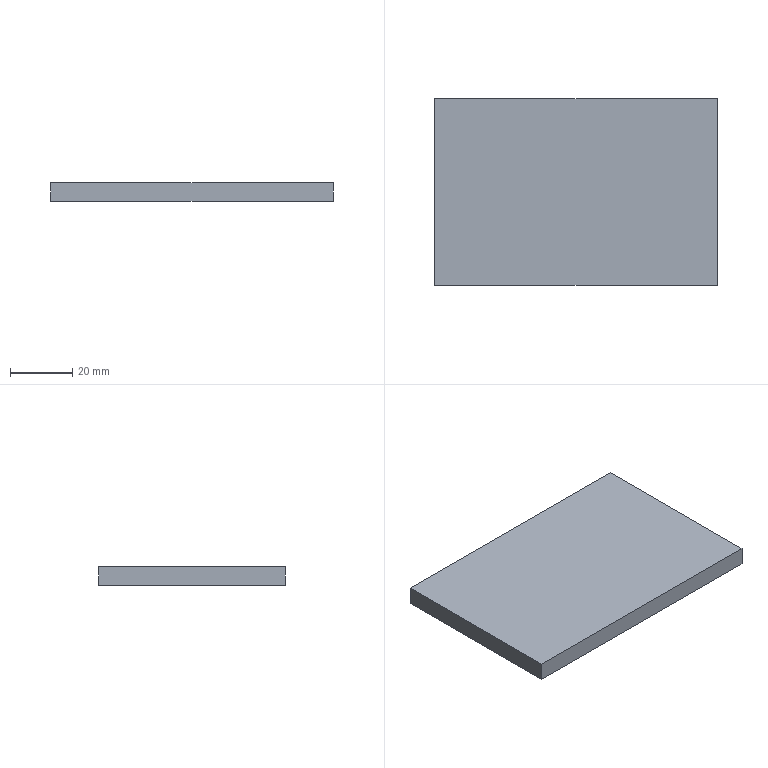Part | STEP file | Plate 3 | 1 solid | 6 faces | box 91 x 60 x 6 mm | volume 32760 mm3 | plane 6
STEP:
#1=CARTESIAN_POINT('',(45.5,-30.,0.));
#2=VERTEX_POINT('',#1);
#3=CARTESIAN_POINT('',(45.5,30.,0.));
#4=VERTEX_POINT('',#3);
#5=CARTESIAN_POINT('',(45.5,-30.,0.));
#6=DIRECTION('',(0.,1.,0.));
#7=VECTOR('',#6,1000.);
#8=LINE('',#5,#7);
#9=EDGE_CURVE('',#2,#4,#8,.T.);
#10=ORIENTED_EDGE('',*,*,#9,.T.);
#11=CARTESIAN_POINT('',(45.5,30.,6.));
#12=VERTEX_POINT('',#11);
#13=CARTESIAN_POINT('',(45.5,30.,6.));
#14=DIRECTION('',(0.,0.,-1.));
#15=VECTOR('',#14,1000.);
#16=LINE('',#13,#15);
#17=EDGE_CURVE('',#12,#4,#16,.T.);
#18=ORIENTED_EDGE('',*,*,#17,.F.);
#19=CARTESIAN_POINT('',(45.5,-30.,6.));
#20=VERTEX_POINT('',#19);
#21=CARTESIAN_POINT('',(45.5,-30.,6.));
#22=DIRECTION('',(0.,1.,0.));
#23=VECTOR('',#22,1000.);
#24=LINE('',#21,#23);
#25=EDGE_CURVE('',#20,#12,#24,.T.);
#26=ORIENTED_EDGE('',*,*,#25,.F.);
#27=CARTESIAN_POINT('',(45.5,-30.,6.));
#28=DIRECTION('',(0.,0.,-1.));
#29=VECTOR('',#28,1000.);
#30=LINE('',#27,#29);
#31=EDGE_CURVE('',#20,#2,#30,.T.);
#32=ORIENTED_EDGE('',*,*,#31,.T.);
#33=EDGE_LOOP('',(#10,#18,#26,#32));
#34=FACE_OUTER_BOUND('',#33,.T.);
#35=CARTESIAN_POINT('',(45.5,-30.,6.));
#36=DIRECTION('',(-1.,0.,0.));
#37=DIRECTION('',(0.,0.,1.));
#38=AXIS2_PLACEMENT_3D('',#35,#36,#37);
#39=PLANE('',#38);
#40=ADVANCED_FACE('',(#34),#39,.F.);
#41=CARTESIAN_POINT('',(-45.5,30.,0.));
#42=VERTEX_POINT('',#41);
#43=CARTESIAN_POINT('',(-45.5,30.,0.));
#44=DIRECTION('',(-1.,0.,0.));
#45=VECTOR('',#44,1000.);
#46=LINE('',#43,#45);
#47=EDGE_CURVE('',#4,#42,#46,.T.);
#48=ORIENTED_EDGE('',*,*,#47,.T.);
#49=CARTESIAN_POINT('',(-45.5,30.,6.));
#50=VERTEX_POINT('',#49);
#51=CARTESIAN_POINT('',(-45.5,30.,6.));
#52=DIRECTION('',(0.,0.,-1.));
#53=VECTOR('',#52,1000.);
#54=LINE('',#51,#53);
#55=EDGE_CURVE('',#50,#42,#54,.T.);
#56=ORIENTED_EDGE('',*,*,#55,.F.);
#57=CARTESIAN_POINT('',(-45.5,30.,6.));
#58=DIRECTION('',(-1.,0.,0.));
#59=VECTOR('',#58,1000.);
#60=LINE('',#57,#59);
#61=EDGE_CURVE('',#12,#50,#60,.T.);
#62=ORIENTED_EDGE('',*,*,#61,.F.);
#63=ORIENTED_EDGE('',*,*,#17,.T.);
#64=EDGE_LOOP('',(#48,#56,#62,#63));
#65=FACE_OUTER_BOUND('',#64,.T.);
#66=CARTESIAN_POINT('',(-45.5,30.,6.));
#67=DIRECTION('',(0.,-1.,0.));
#68=DIRECTION('',(0.,0.,-1.));
#69=AXIS2_PLACEMENT_3D('',#66,#67,#68);
#70=PLANE('',#69);
#71=ADVANCED_FACE('',(#65),#70,.F.);
#72=CARTESIAN_POINT('',(-45.5,-30.,0.));
#73=VERTEX_POINT('',#72);
#74=CARTESIAN_POINT('',(-45.5,-30.,0.));
#75=DIRECTION('',(0.,-1.,0.));
#76=VECTOR('',#75,1000.);
#77=LINE('',#74,#76);
#78=EDGE_CURVE('',#42,#73,#77,.T.);
#79=ORIENTED_EDGE('',*,*,#78,.T.);
#80=CARTESIAN_POINT('',(-45.5,-30.,6.));
#81=VERTEX_POINT('',#80);
#82=CARTESIAN_POINT('',(-45.5,-30.,6.));
#83=DIRECTION('',(0.,0.,-1.));
#84=VECTOR('',#83,1000.);
#85=LINE('',#82,#84);
#86=EDGE_CURVE('',#81,#73,#85,.T.);
#87=ORIENTED_EDGE('',*,*,#86,.F.);
#88=CARTESIAN_POINT('',(-45.5,-30.,6.));
#89=DIRECTION('',(0.,-1.,0.));
#90=VECTOR('',#89,1000.);
#91=LINE('',#88,#90);
#92=EDGE_CURVE('',#50,#81,#91,.T.);
#93=ORIENTED_EDGE('',*,*,#92,.F.);
#94=ORIENTED_EDGE('',*,*,#55,.T.);
#95=EDGE_LOOP('',(#79,#87,#93,#94));
#96=FACE_OUTER_BOUND('',#95,.T.);
#97=CARTESIAN_POINT('',(-45.5,-30.,6.));
#98=DIRECTION('',(1.,0.,0.));
#99=DIRECTION('',(0.,0.,-1.));
#100=AXIS2_PLACEMENT_3D('',#97,#98,#99);
#101=PLANE('',#100);
#102=ADVANCED_FACE('',(#96),#101,.F.);
#103=CARTESIAN_POINT('',(-45.5,-30.,0.));
#104=DIRECTION('',(1.,0.,0.));
#105=VECTOR('',#104,1000.);
#106=LINE('',#103,#105);
#107=EDGE_CURVE('',#73,#2,#106,.T.);
#108=ORIENTED_EDGE('',*,*,#107,.T.);
#109=ORIENTED_EDGE('',*,*,#31,.F.);
#110=CARTESIAN_POINT('',(-45.5,-30.,6.));
#111=DIRECTION('',(1.,0.,0.));
#112=VECTOR('',#111,1000.);
#113=LINE('',#110,#112);
#114=EDGE_CURVE('',#81,#20,#113,.T.);
#115=ORIENTED_EDGE('',*,*,#114,.F.);
#116=ORIENTED_EDGE('',*,*,#86,.T.);
#117=EDGE_LOOP('',(#108,#109,#115,#116));
#118=FACE_OUTER_BOUND('',#117,.T.);
#119=CARTESIAN_POINT('',(-45.5,-30.,6.));
#120=DIRECTION('',(0.,1.,0.));
#121=DIRECTION('',(0.,0.,1.));
#122=AXIS2_PLACEMENT_3D('',#119,#120,#121);
#123=PLANE('',#122);
#124=ADVANCED_FACE('',(#118),#123,.F.);
#125=ORIENTED_EDGE('',*,*,#25,.T.);
#126=ORIENTED_EDGE('',*,*,#61,.T.);
#127=ORIENTED_EDGE('',*,*,#92,.T.);
#128=ORIENTED_EDGE('',*,*,#114,.T.);
#129=EDGE_LOOP('',(#125,#126,#127,#128));
#130=FACE_OUTER_BOUND('',#129,.T.);
#131=CARTESIAN_POINT('',(0.,0.,6.));
#132=DIRECTION('',(0.,0.,-1.));
#133=DIRECTION('',(-1.,0.,0.));
#134=AXIS2_PLACEMENT_3D('',#131,#132,#133);
#135=PLANE('',#134);
#136=ADVANCED_FACE('',(#130),#135,.F.);
#137=ORIENTED_EDGE('',*,*,#9,.F.);
#138=ORIENTED_EDGE('',*,*,#107,.F.);
#139=ORIENTED_EDGE('',*,*,#78,.F.);
#140=ORIENTED_EDGE('',*,*,#47,.F.);
#141=EDGE_LOOP('',(#137,#138,#139,#140));
#142=FACE_OUTER_BOUND('',#141,.T.);
#143=CARTESIAN_POINT('',(0.,0.,0.));
#144=DIRECTION('',(0.,0.,-1.));
#145=DIRECTION('',(-1.,0.,0.));
#146=AXIS2_PLACEMENT_3D('',#143,#144,#145);
#147=PLANE('',#146);
#148=ADVANCED_FACE('',(#142),#147,.T.);
#149=CLOSED_SHELL('',(#40,#71,#102,#124,#136,#148));
#150=MANIFOLD_SOLID_BREP('',#149);
#151=CARTESIAN_POINT('',(0.,0.,0.));
#152=DIRECTION('',(0.,0.,1.));
#153=DIRECTION('',(1.,0.,0.));
#154=AXIS2_PLACEMENT_3D('',#151,#152,#153);
#155=(LENGTH_UNIT()NAMED_UNIT(*)SI_UNIT(.MILLI.,.METRE.));
#156=UNCERTAINTY_MEASURE_WITH_UNIT(LENGTH_MEASURE(0.00001),#155,'','');
#157=(NAMED_UNIT(*)PLANE_ANGLE_UNIT()SI_UNIT($,.RADIAN.));
#158=(NAMED_UNIT(*)SI_UNIT($,.STERADIAN.)SOLID_ANGLE_UNIT());
#159=(GEOMETRIC_REPRESENTATION_CONTEXT(3)GLOBAL_UNCERTAINTY_ASSIGNED_CONTEXT((#156))GLOBAL_UNIT_ASSIGNED_CONTEXT((#155,#157,#158))REPRESENTATION_CONTEXT('',''));
#160=ADVANCED_BREP_SHAPE_REPRESENTATION('',(#150,#154),#159);